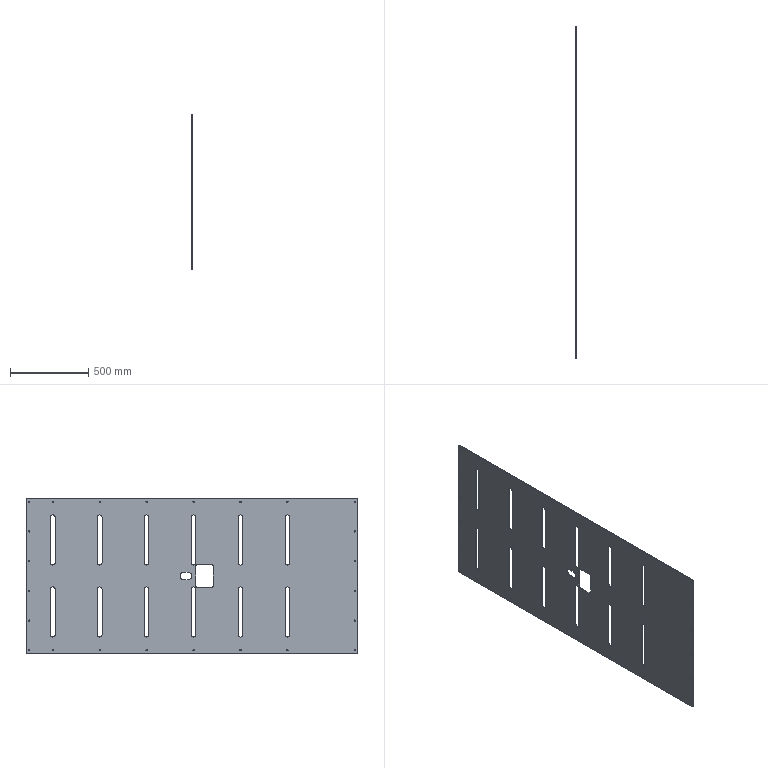Part | SolidWorks | features LPattern 7, ICE 5, MirrorPattern 4, Fillet 2, HoleWzd 2, Extrusion 1 | 1 solid | 130 faces | box 5 x 2120 x 990 mm | volume 9826354 mm3 | cylinder 94 | plane 36 | commonest cylinder face diameters 8 x48 30 x36 20 x8 45 x2